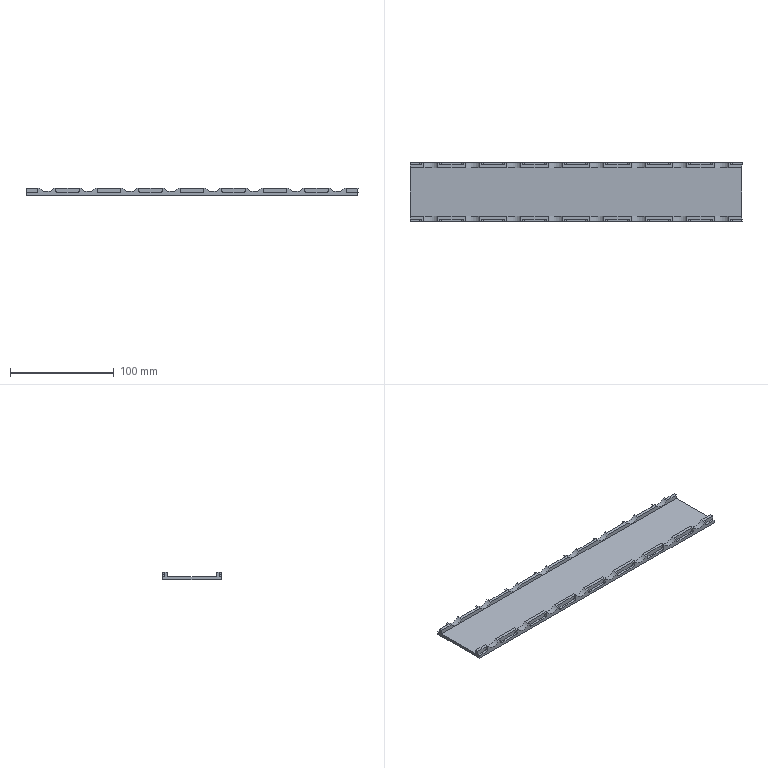NC program | Mastercam | posted with a generic post
Lines 4971 to 6130 of 9376:
(2 BM/BNOS |TOOL - 5|DIA. OFF. - 5|LEN. - 5|TOOL DIA. - 2.)
N104 T5 M6
N106 G0 G54 G90 X13.026 Y21.528 C0. B0. S6000 M3
N108 G43 H5 Z50.
N110 Z28.438
N112 Z11.438
N114 G1 Z8.438 F2000.
N116 Y21.544 Z8.246 F1000.
N118 Y21.588 Z8.058
N120 Y21.656 Z7.873
N122 Y21.745 Z7.695
N124 Y21.852 Z7.523
N126 Y21.971 Z7.36
N128 Y22.236 Z7.064
N130 X12.999 Y22.337 Z6.963
N132 X12.926 Y22.429 Z6.871
N134 X12.815 Y22.509 Z6.791
N136 X12.676 Y22.577 Z6.723
N138 X12.518 Y22.632 Z6.668
N140 X12.351 Y22.673 Z6.627
N142 X12.184 Y22.698 Z6.602
N144 X12.026 Y22.707 Z6.593
N146 X11.026
N148 X10.855
N150 X9.407
N152 X7.96
N154 X6.513
N156 X5.066
N158 X3.618
N160 X2.171
N162 X.724
N164 X-.724
N166 X-2.171
N168 X-3.618
N170 X-5.066
N172 X-6.513
N174 X-7.96
N176 X-9.407
N178 X-10.855
N180 X-12.302
N182 X-13.026
N184 X-13.057 Z6.592
N186 X-13.088 Z6.59
N188 X-13.118 Z6.586
N190 X-13.149 Z6.58
N192 X-13.179 Z6.573
N194 X-13.209 Z6.564
N196 X-13.238 Z6.554
N198 X-13.267 Z6.542
N200 X-13.295 Z6.529
N202 X-13.322 Z6.514
N204 X-13.348 Z6.498
N206 X-13.374 Z6.48
N208 X-13.398 Z6.461
N210 X-13.422 Z6.441
N212 X-13.445 Z6.42
N214 X-13.466 Z6.397
N216 X-13.599 Z6.251
N218 X-13.86 Z5.973
N220 X-14.123 Z5.717
N222 X-14.397 Z5.472
N224 X-14.681 Z5.239
N226 X-14.974 Z5.018
N228 X-15.277 Z4.81
N230 X-15.588 Z4.615
N232 X-15.907 Z4.432
N234 X-16.246 Z4.258
N236 X-16.592 Z4.099
N238 X-16.933 Z3.962
N240 X-17.279 Z3.839
N242 X-17.63 Z3.73
N244 X-17.985 Z3.637
N246 X-18.344 Z3.559
N248 X-18.706 Z3.495
N250 X-19.07 Z3.447
N252 X-19.435 Z3.415
N254 X-19.802 Z3.398
N256 X-20.184
N258 X-20.565 Z3.415
N260 X-20.93 Z3.447
N262 X-21.294 Z3.495
N264 X-21.656 Z3.559
N266 X-22.015 Z3.637
N268 X-22.37 Z3.73
N270 X-22.721 Z3.839
N272 X-23.067 Z3.962
N274 X-23.408 Z4.099
N276 X-23.754 Z4.258
N278 X-24.093 Z4.432
N280 X-24.412 Z4.615
N282 X-24.723 Z4.81
N284 X-25.026 Z5.018
N286 X-25.319 Z5.239
N288 X-25.603 Z5.472
N290 X-25.877 Z5.717
N292 X-26.14 Z5.973
N294 X-26.401 Z6.251
N296 X-26.534 Z6.397
N298 X-26.555 Z6.42
N300 X-26.578 Z6.441
N302 X-26.602 Z6.461
N304 X-26.626 Z6.48
N306 X-26.652 Z6.498
N308 X-26.678 Z6.514
N310 X-26.705 Z6.529
N312 X-26.733 Z6.542
N314 X-26.762 Z6.554
N316 X-26.791 Z6.564
N318 X-26.821 Z6.573
N320 X-26.851 Z6.58
N322 X-26.882 Z6.586
N324 X-26.912 Z6.59
N326 X-26.943 Z6.592
N328 X-26.974 Z6.593
N330 X-27.698
N332 X-29.145
N334 X-30.593
N336 X-32.04
N338 X-33.487
N340 X-34.934
N342 X-36.382
N344 X-37.829
N346 X-39.276
N348 X-40.724
N350 X-42.171
N352 X-43.618
N354 X-45.066
N356 X-46.513
N358 X-47.96
N360 X-49.407
N362 X-50.855
N364 X-52.302
N366 X-53.026
N368 X-53.057 Z6.592
N370 X-53.088 Z6.59
N372 X-53.118 Z6.586
N374 X-53.149 Z6.58
N376 X-53.179 Z6.573
N378 X-53.209 Z6.564
N380 X-53.238 Z6.554
N382 X-53.267 Z6.542
N384 X-53.295 Z6.529
N386 X-53.322 Z6.514
N388 X-53.348 Z6.498
N390 X-53.374 Z6.48
N392 X-53.398 Z6.461
N394 X-53.422 Z6.441
N396 X-53.445 Z6.42
N398 X-53.466 Z6.397
N400 X-53.599 Z6.251
N402 X-53.86 Z5.973
N404 X-54.123 Z5.717
N406 X-54.397 Z5.472
N408 X-54.681 Z5.239
N410 X-54.974 Z5.018
N412 X-55.277 Z4.81
N414 X-55.588 Z4.615
N416 X-55.907 Z4.432
N418 X-56.246 Z4.258
N420 X-56.592 Z4.099
N422 X-56.933 Z3.962
N424 X-57.279 Z3.839
N426 X-57.63 Z3.73
N428 X-57.985 Z3.637
N430 X-58.344 Z3.559
N432 X-58.706 Z3.495
N434 X-59.07 Z3.447
N436 X-59.435 Z3.415
N438 X-59.802 Z3.398
N440 X-60.184
N442 X-60.565 Z3.415
N444 X-60.93 Z3.447
N446 X-61.294 Z3.495
N448 X-61.656 Z3.559
N450 X-62.015 Z3.637
N452 X-62.37 Z3.73
N454 X-62.721 Z3.839
N456 X-63.067 Z3.962
N458 X-63.408 Z4.099
N460 X-63.754 Z4.258
N462 X-64.093 Z4.432
N464 X-64.412 Z4.615
N466 X-64.723 Z4.81
N468 X-65.026 Z5.018
N470 X-65.319 Z5.239
N472 X-65.603 Z5.472
N474 X-65.877 Z5.717
N476 X-66.14 Z5.973
N478 X-66.401 Z6.251
N480 X-66.534 Z6.397
N482 X-66.555 Z6.42
N484 X-66.578 Z6.441
N486 X-66.602 Z6.461
N488 X-66.626 Z6.48
N490 X-66.652 Z6.498
N492 X-66.678 Z6.514
N494 X-66.705 Z6.529
N496 X-66.733 Z6.542
N498 X-66.762 Z6.554
N500 X-66.791 Z6.564
N502 X-66.821 Z6.573
N504 X-66.851 Z6.58
N506 X-66.882 Z6.586
N508 X-66.912 Z6.59
N510 X-66.943 Z6.592
N512 X-66.974 Z6.593
N514 X-67.698
N516 X-69.145
N518 X-70.593
N520 X-72.04
N522 X-73.487
N524 X-74.934
N526 X-76.382
N528 X-77.829
N530 X-79.276
N532 X-80.724
N534 X-82.171
N536 X-83.618
N538 X-85.066
N540 X-86.513
N542 X-87.96
N544 X-89.407
N546 X-90.855
N548 X-92.302
N550 X-93.026
N552 X-93.057 Z6.592
N554 X-93.088 Z6.59
N556 X-93.118 Z6.586
N558 X-93.149 Z6.58
N560 X-93.179 Z6.573
N562 X-93.209 Z6.564
N564 X-93.238 Z6.554
N566 X-93.267 Z6.542
N568 X-93.295 Z6.529
N570 X-93.322 Z6.514
N572 X-93.348 Z6.498
N574 X-93.374 Z6.48
N576 X-93.398 Z6.461
N578 X-93.422 Z6.441
N580 X-93.445 Z6.42
N582 X-93.466 Z6.397
N584 X-93.599 Z6.251
N586 X-93.86 Z5.973
N588 X-94.123 Z5.717
N590 X-94.397 Z5.472
N592 X-94.681 Z5.239
N594 X-94.974 Z5.018
N596 X-95.277 Z4.81
N598 X-95.588 Z4.615
N600 X-95.907 Z4.432
N602 X-96.246 Z4.258
N604 X-96.592 Z4.099
N606 X-96.933 Z3.962
N608 X-97.279 Z3.839
N610 X-97.63 Z3.73
N612 X-97.985 Z3.637
N614 X-98.344 Z3.559
N616 X-98.706 Z3.495
N618 X-99.07 Z3.447
N620 X-99.435 Z3.415
N622 X-99.816 Z3.398
N624 X-100.198
N626 X-100.565 Z3.415
N628 X-100.93 Z3.447
N630 X-101.294 Z3.495
N632 X-101.656 Z3.559
N634 X-102.015 Z3.637
N636 X-102.37 Z3.73
N638 X-102.721 Z3.839
N640 X-103.067 Z3.962
N642 X-103.408 Z4.099
N644 X-103.754 Z4.258
N646 X-104.093 Z4.432
N648 X-104.412 Z4.615
N650 X-104.723 Z4.81
N652 X-105.026 Z5.018
N654 X-105.319 Z5.239
N656 X-105.603 Z5.472
N658 X-105.877 Z5.717
N660 X-106.14 Z5.973
N662 X-106.401 Z6.251
N664 X-106.534 Z6.397
N666 X-106.555 Z6.42
N668 X-106.578 Z6.441
N670 X-106.602 Z6.461
N672 X-106.626 Z6.48
N674 X-106.652 Z6.498
N676 X-106.678 Z6.514
N678 X-106.705 Z6.529
N680 X-106.733 Z6.542
N682 X-106.762 Z6.554
N684 X-106.791 Z6.564
N686 X-106.821 Z6.573
N688 X-106.851 Z6.58
N690 X-106.882 Z6.586
N692 X-106.912 Z6.59
N694 X-106.943 Z6.592
N696 X-106.974 Z6.593
N698 X-107.698
N700 X-109.145
N702 X-110.593
N704 X-112.04
N706 X-113.487
N708 X-114.934
N710 X-116.382
N712 X-117.829
N714 X-119.276
N716 X-120.724
N718 X-122.171
N720 X-123.618
N722 X-125.066
N724 X-126.513
N726 X-127.96
N728 X-129.408
N730 X-130.855
N732 X-132.302
N734 X-133.026
N736 X-133.057 Z6.592
N738 X-133.088 Z6.59
N740 X-133.118 Z6.586
N742 X-133.149 Z6.58
N744 X-133.179 Z6.573
N746 X-133.209 Z6.564
N748 X-133.238 Z6.554
N750 X-133.267 Z6.542
N752 X-133.295 Z6.529
N754 X-133.322 Z6.514
N756 X-133.348 Z6.498
N758 X-133.374 Z6.48
N760 X-133.398 Z6.461
N762 X-133.422 Z6.441
N764 X-133.445 Z6.42
N766 X-133.466 Z6.397
N768 X-133.599 Z6.251
N770 X-133.86 Z5.973
N772 X-134.123 Z5.717
N774 X-134.397 Z5.472
N776 X-134.681 Z5.239
N778 X-134.974 Z5.018
N780 X-135.277 Z4.81
N782 X-135.588 Z4.615
N784 X-135.907 Z4.432
N786 X-136.246 Z4.258
N788 X-136.592 Z4.099
N790 X-136.933 Z3.962
N792 X-137.279 Z3.839
N794 X-137.63 Z3.73
N796 X-137.985 Z3.637
N798 X-138.344 Z3.559
N800 X-138.706 Z3.495
N802 X-139.07 Z3.447
N804 X-139.435 Z3.415
N806 X-139.802 Z3.398
N808 X-140.184
N810 X-140.565 Z3.415
N812 X-140.93 Z3.447
N814 X-141.294 Z3.495
N816 X-141.656 Z3.559
N818 X-142.015 Z3.637
N820 X-142.37 Z3.73
N822 X-142.721 Z3.839
N824 X-143.067 Z3.962
N826 X-143.408 Z4.099
N828 X-143.754 Z4.258
N830 X-144.093 Z4.432
N832 X-144.412 Z4.615
N834 X-144.723 Z4.81
N836 X-145.026 Z5.018
N838 X-145.319 Z5.239
N840 X-145.603 Z5.472
N842 X-145.877 Z5.717
N844 X-146.14 Z5.973
N846 X-146.401 Z6.251
N848 X-146.534 Z6.397
N850 X-146.555 Z6.42
N852 X-146.578 Z6.441
N854 X-146.602 Z6.461
N856 X-146.626 Z6.48
N858 X-146.652 Z6.498
N860 X-146.678 Z6.514
N862 X-146.705 Z6.529
N864 X-146.733 Z6.542
N866 X-146.762 Z6.554
N868 X-146.791 Z6.564
N870 X-146.821 Z6.573
N872 X-146.851 Z6.58
N874 X-146.882 Z6.586
N876 X-146.912 Z6.59
N878 X-146.943 Z6.592
N880 X-146.974 Z6.593
N882 X-147.698
N884 X-149.145
N886 X-150.593
N888 X-152.04
N890 X-153.487
N892 X-154.934
N894 X-156.382
N896 X-157.829
N898 X-159.276
N900 X-160.
N902 X-160.031 Y22.708
N904 X-160.062 Y22.71
N906 X-160.093 Y22.714
N908 X-160.123 Y22.72
N910 X-160.153 Y22.727
N912 X-160.183 Y22.736
N914 X-160.213 Y22.746
N916 X-160.241 Y22.758
N918 X-160.269 Y22.772
N920 X-160.297 Y22.786
N922 X-160.323 Y22.803
N924 X-160.349 Y22.82
N926 X-160.373 Y22.839
N928 X-160.397 Y22.859
N930 X-160.419 Y22.881
N932 X-160.441 Y22.903
N934 X-160.461 Y22.927
N936 X-160.48 Y22.951
N938 X-160.497 Y22.977
N940 X-160.514 Y23.003
N942 X-160.528 Y23.031
N944 X-160.542 Y23.059
N946 X-160.554 Y23.087
N948 X-160.564 Y23.117
N950 X-160.573 Y23.147
N952 X-160.58 Y23.177
N954 X-160.586 Y23.207
N956 X-160.59 Y23.238
N958 X-160.592 Y23.269
N960 X-160.593 Y23.3
N962 Y24.
N964 Y25.4
N966 Y26.1
N968 X-160.592 Y26.131
N970 X-160.59 Y26.162
N972 X-160.586 Y26.193
N974 X-160.58 Y26.223
N976 X-160.573 Y26.253
N978 X-160.564 Y26.283
N980 X-160.554 Y26.313
N982 X-160.542 Y26.341
N984 X-160.528 Y26.369
N986 X-160.514 Y26.397
N988 X-160.497 Y26.423
N990 X-160.48 Y26.449
N992 X-160.461 Y26.473
N994 X-160.441 Y26.497
N996 X-160.419 Y26.519
N998 X-160.397 Y26.541
N1000 X-160.373 Y26.561
N1002 X-160.349 Y26.58
N1004 X-160.323 Y26.597
N1006 X-160.297 Y26.614
N1008 X-160.269 Y26.628
N1010 X-160.241 Y26.642
N1012 X-160.213 Y26.654
N1014 X-160.183 Y26.664
N1016 X-160.153 Y26.673
N1018 X-160.123 Y26.68
N1020 X-160.093 Y26.686
N1022 X-160.062 Y26.69
N1024 X-160.031 Y26.692
N1026 X-160. Y26.693
N1028 X-159.281
N1030 X-157.844
N1032 X-156.406
N1034 X-154.969
N1036 X-153.531
N1038 X-152.094
N1040 X-150.656
N1042 X-149.219
N1044 X-149.093
N1046 Y27.75
N1048 Y28.3
N1050 X-149.092 Y28.331
N1052 X-149.09 Y28.362
N1054 X-149.086 Y28.393
N1056 X-149.08 Y28.423
N1058 X-149.073 Y28.453
N1060 X-149.064 Y28.483
N1062 X-149.054 Y28.513
N1064 X-149.042 Y28.541
N1066 X-149.028 Y28.569
N1068 X-149.014 Y28.597
N1070 X-148.997 Y28.623
N1072 X-148.98 Y28.649
N1074 X-148.961 Y28.673
N1076 X-148.941 Y28.697
N1078 X-148.919 Y28.719
N1080 X-148.897 Y28.741
N1082 X-148.873 Y28.761
N1084 X-148.849 Y28.78
N1086 X-148.823 Y28.797
N1088 X-148.797 Y28.814
N1090 X-148.769 Y28.828
N1092 X-148.741 Y28.842
N1094 X-148.713 Y28.854
N1096 X-148.683 Y28.864
N1098 X-148.653 Y28.873
N1100 X-148.623 Y28.88
N1102 X-148.593 Y28.886
N1104 X-148.562 Y28.89
N1106 X-148.531 Y28.892
N1108 X-148.5 Y28.893
N1110 X-148.119
N1112 X-147.356
N1114 X-146.974
N1116 X-146.943 Z6.592
N1118 X-146.912 Z6.59
N1120 X-146.882 Z6.586
N1122 X-146.851 Z6.58
N1124 X-146.821 Z6.573
N1126 X-146.791 Z6.564
N1128 X-146.762 Z6.554
N1130 X-146.733 Z6.542
N1132 X-146.705 Z6.529
N1134 X-146.678 Z6.514
N1136 X-146.652 Z6.498
N1138 X-146.626 Z6.48
N1140 X-146.602 Z6.461
N1142 X-146.578 Z6.441
N1144 X-146.555 Z6.42
N1146 X-146.534 Z6.397
N1148 X-146.401 Z6.251
N1150 X-146.14 Z5.973
N1152 X-145.877 Z5.717
N1154 X-145.603 Z5.472
N1156 X-145.319 Z5.239
N1158 X-145.026 Z5.018
N1160 X-144.723 Z4.81
N1162 X-144.412 Z4.615
N1164 X-144.093 Z4.432
N1166 X-143.754 Z4.258
N1168 X-143.408 Z4.099
N1170 X-143.067 Z3.962
N1172 X-142.721 Z3.839
N1174 X-142.37 Z3.73
N1176 X-142.015 Z3.637
N1178 X-141.656 Z3.559
N1180 X-141.294 Z3.495
N1182 X-140.93 Z3.447
N1184 X-140.565 Z3.415
N1186 X-140.184 Z3.398
N1188 X-139.802
N1190 X-139.435 Z3.415
N1192 X-139.07 Z3.447
N1194 X-138.706 Z3.495
N1196 X-138.344 Z3.559
N1198 X-137.985 Z3.637
N1200 X-137.63 Z3.73
N1202 X-137.279 Z3.839
N1204 X-136.933 Z3.962
N1206 X-136.592 Z4.099
N1208 X-136.246 Z4.258
N1210 X-135.907 Z4.432
N1212 X-135.588 Z4.615
N1214 X-135.277 Z4.81
N1216 X-134.974 Z5.018
N1218 X-134.681 Z5.239
N1220 X-134.397 Z5.472
N1222 X-134.123 Z5.717
N1224 X-133.86 Z5.973
N1226 X-133.599 Z6.251
N1228 X-133.466 Z6.397
N1230 X-133.445 Z6.42
N1232 X-133.422 Z6.441
N1234 X-133.398 Z6.461
N1236 X-133.374 Z6.48
N1238 X-133.348 Z6.498
N1240 X-133.322 Z6.514
N1242 X-133.295 Z6.529
N1244 X-133.267 Z6.542
N1246 X-133.238 Z6.554
N1248 X-133.209 Z6.564
N1250 X-133.179 Z6.573
N1252 X-133.149 Z6.58
N1254 X-133.118 Z6.586
N1256 X-133.088 Z6.59
N1258 X-133.057 Z6.592
N1260 X-133.026 Z6.593
N1262 X-132.644
N1264 X-131.881
N1266 X-131.5
N1268 X-131.469 Y28.892
N1270 X-131.438 Y28.89
N1272 X-131.407 Y28.886
N1274 X-131.377 Y28.88
N1276 X-131.347 Y28.873
N1278 X-131.317 Y28.864
N1280 X-131.287 Y28.854
N1282 X-131.259 Y28.842
N1284 X-131.231 Y28.828
N1286 X-131.203 Y28.814
N1288 X-131.177 Y28.797
N1290 X-131.151 Y28.78
N1292 X-131.127 Y28.761
N1294 X-131.103 Y28.741
N1296 X-131.081 Y28.719
N1298 X-131.059 Y28.697
N1300 X-131.039 Y28.673
N1302 X-131.02 Y28.649
N1304 X-131.003 Y28.623
N1306 X-130.986 Y28.597
N1308 X-130.972 Y28.569
N1310 X-130.958 Y28.541
N1312 X-130.946 Y28.513
N1314 X-130.936 Y28.483
N1316 X-130.927 Y28.453
N1318 X-130.92 Y28.423
N1320 X-130.914 Y28.393
N1322 X-130.91 Y28.362
N1324 X-130.908 Y28.331
N1326 X-130.907 Y28.3
N1328 Y27.75
N1330 Y26.693
N1332 X-130.781
N1334 X-129.344
N1336 X-127.906
N1338 X-126.469
N1340 X-125.031
N1342 X-123.594
N1344 X-122.156
N1346 X-120.719
N1348 X-119.281
N1350 X-117.844
N1352 X-116.406
N1354 X-114.969
N1356 X-113.531
N1358 X-112.094
N1360 X-110.656
N1362 X-109.219
N1364 X-109.093
N1366 Y27.75
N1368 Y28.3
N1370 X-109.092 Y28.331
N1372 X-109.09 Y28.362
N1374 X-109.086 Y28.393
N1376 X-109.08 Y28.423
N1378 X-109.073 Y28.453
N1380 X-109.064 Y28.483
N1382 X-109.054 Y28.513
N1384 X-109.042 Y28.541
N1386 X-109.028 Y28.569
N1388 X-109.014 Y28.597
N1390 X-108.997 Y28.623
N1392 X-108.98 Y28.649
N1394 X-108.961 Y28.673
N1396 X-108.941 Y28.697
N1398 X-108.919 Y28.719
N1400 X-108.897 Y28.741
N1402 X-108.873 Y28.761
N1404 X-108.849 Y28.78
N1406 X-108.823 Y28.797
N1408 X-108.797 Y28.814
N1410 X-108.769 Y28.828
N1412 X-108.741 Y28.842
N1414 X-108.713 Y28.854
N1416 X-108.683 Y28.864
N1418 X-108.653 Y28.873
N1420 X-108.623 Y28.88
N1422 X-108.593 Y28.886
N1424 X-108.562 Y28.89
N1426 X-108.531 Y28.892
N1428 X-108.5 Y28.893
N1430 X-108.119
N1432 X-107.356
N1434 X-106.974
N1436 X-106.943 Z6.592
N1438 X-106.912 Z6.59
N1440 X-106.882 Z6.586
N1442 X-106.851 Z6.58
N1444 X-106.821 Z6.573
N1446 X-106.791 Z6.564
N1448 X-106.762 Z6.554
N1450 X-106.733 Z6.542
N1452 X-106.705 Z6.529
N1454 X-106.678 Z6.514
N1456 X-106.652 Z6.498
N1458 X-106.626 Z6.48
N1460 X-106.602 Z6.461
N1462 X-106.578 Z6.441
N1464 X-106.555 Z6.42
N1466 X-106.534 Z6.397
N1468 X-106.401 Z6.251
N1470 X-106.14 Z5.973
N1472 X-105.877 Z5.717
N1474 X-105.603 Z5.472
N1476 X-105.319 Z5.239
N1478 X-105.026 Z5.018
N1480 X-104.723 Z4.81
N1482 X-104.412 Z4.615
N1484 X-104.093 Z4.432
N1486 X-103.754 Z4.258
N1488 X-103.408 Z4.099
N1490 X-103.067 Z3.962
N1492 X-102.721 Z3.839
N1494 X-102.37 Z3.73
N1496 X-102.015 Z3.637
N1498 X-101.656 Z3.559
N1500 X-101.294 Z3.495
N1502 X-100.93 Z3.447
N1504 X-100.565 Z3.415
N1506 X-100.198 Z3.398
N1508 X-99.816
N1510 X-99.435 Z3.415
N1512 X-99.07 Z3.447
N1514 X-98.706 Z3.495
N1516 X-98.344 Z3.559
N1518 X-97.985 Z3.637
N1520 X-97.63 Z3.73
N1522 X-97.279 Z3.839
N1524 X-96.933 Z3.962
N1526 X-96.592 Z4.099
N1528 X-96.246 Z4.258
N1530 X-95.907 Z4.432
N1532 X-95.588 Z4.615
N1534 X-95.277 Z4.81
N1536 X-94.974 Z5.018
N1538 X-94.681 Z5.239
N1540 X-94.397 Z5.472
N1542 X-94.123 Z5.717
N1544 X-93.86 Z5.973
N1546 X-93.599 Z6.251
N1548 X-93.466 Z6.397
N1550 X-93.445 Z6.42
N1552 X-93.422 Z6.441
N1554 X-93.398 Z6.461
N1556 X-93.374 Z6.48
N1558 X-93.348 Z6.498
N1560 X-93.322 Z6.514
N1562 X-93.295 Z6.529
N1564 X-93.267 Z6.542
N1566 X-93.238 Z6.554
N1568 X-93.209 Z6.564
N1570 X-93.179 Z6.573
N1572 X-93.149 Z6.58
N1574 X-93.118 Z6.586
N1576 X-93.088 Z6.59
N1578 X-93.057 Z6.592
N1580 X-93.026 Z6.593
N1582 X-92.644
N1584 X-91.881
N1586 X-91.5
N1588 X-91.469 Y28.892
N1590 X-91.438 Y28.89
N1592 X-91.407 Y28.886
N1594 X-91.377 Y28.88
N1596 X-91.347 Y28.873
N1598 X-91.317 Y28.864
N1600 X-91.287 Y28.854
N1602 X-91.259 Y28.842
N1604 X-91.231 Y28.828
N1606 X-91.203 Y28.814
N1608 X-91.177 Y28.797
N1610 X-91.151 Y28.78
N1612 X-91.127 Y28.761
N1614 X-91.103 Y28.741
N1616 X-91.081 Y28.719
N1618 X-91.059 Y28.697
N1620 X-91.039 Y28.673
N1622 X-91.02 Y28.649
N1624 X-91.003 Y28.623
N1626 X-90.986 Y28.597
N1628 X-90.972 Y28.569
N1630 X-90.958 Y28.541
N1632 X-90.946 Y28.513
N1634 X-90.936 Y28.483
N1636 X-90.927 Y28.453
N1638 X-90.92 Y28.423
N1640 X-90.914 Y28.393
N1642 X-90.91 Y28.362
N1644 X-90.908 Y28.331
N1646 X-90.907 Y28.3
N1648 Y27.75
N1650 Y26.693
N1652 X-90.781
N1654 X-89.344
N1656 X-87.906
N1658 X-86.469
N1660 X-85.031
N1662 X-83.594
N1664 X-82.156
N1666 X-80.719
N1668 X-79.281
N1670 X-77.844
N1672 X-76.406
N1674 X-74.969
N1676 X-73.531
N1678 X-72.094
N1680 X-70.656
N1682 X-69.219
N1684 X-69.093
N1686 Y27.75
N1688 Y28.3
N1690 X-69.092 Y28.331
N1692 X-69.09 Y28.362
N1694 X-69.086 Y28.393
N1696 X-69.08 Y28.423
N1698 X-69.073 Y28.453
N1700 X-69.064 Y28.483
N1702 X-69.054 Y28.513
N1704 X-69.042 Y28.541
N1706 X-69.028 Y28.569
N1708 X-69.014 Y28.597
N1710 X-68.997 Y28.623
N1712 X-68.98 Y28.649
N1714 X-68.961 Y28.673
N1716 X-68.941 Y28.697
N1718 X-68.919 Y28.719
N1720 X-68.897 Y28.741
N1722 X-68.873 Y28.761
N1724 X-68.849 Y28.78
N1726 X-68.823 Y28.797
N1728 X-68.797 Y28.814
N1730 X-68.769 Y28.828
N1732 X-68.741 Y28.842
N1734 X-68.713 Y28.854
N1736 X-68.683 Y28.864
N1738 X-68.653 Y28.873
N1740 X-68.623 Y28.88
N1742 X-68.593 Y28.886
N1744 X-68.562 Y28.89
N1746 X-68.531 Y28.892
N1748 X-68.5 Y28.893
N1750 X-68.119
N1752 X-67.356
N1754 X-66.974
N1756 X-66.943 Z6.592
N1758 X-66.912 Z6.59
N1760 X-66.882 Z6.586
N1762 X-66.851 Z6.58
N1764 X-66.821 Z6.573
N1766 X-66.791 Z6.564
N1768 X-66.762 Z6.554
N1770 X-66.733 Z6.542
N1772 X-66.705 Z6.529
N1774 X-66.678 Z6.514
N1776 X-66.652 Z6.498
N1778 X-66.626 Z6.48
N1780 X-66.602 Z6.461
N1782 X-66.578 Z6.441
N1784 X-66.555 Z6.42
N1786 X-66.534 Z6.397
N1788 X-66.401 Z6.251
N1790 X-66.14 Z5.973
N1792 X-65.877 Z5.717
N1794 X-65.603 Z5.472
N1796 X-65.319 Z5.239
N1798 X-65.026 Z5.018
N1800 X-64.723 Z4.81
N1802 X-64.412 Z4.615
N1804 X-64.093 Z4.432
N1806 X-63.754 Z4.258
N1808 X-63.408 Z4.099
N1810 X-63.067 Z3.962
N1812 X-62.721 Z3.839
N1814 X-62.37 Z3.73
N1816 X-62.015 Z3.637
N1818 X-61.656 Z3.559
N1820 X-61.294 Z3.495
N1822 X-60.93 Z3.447
N1824 X-60.565 Z3.415
N1826 X-60.184 Z3.398
N1828 X-59.802
N1830 X-59.435 Z3.415
N1832 X-59.07 Z3.447
N1834 X-58.706 Z3.495
N1836 X-58.344 Z3.559
N1838 X-57.985 Z3.637
N1840 X-57.63 Z3.73
N1842 X-57.279 Z3.839
N1844 X-56.933 Z3.962
N1846 X-56.592 Z4.099
N1848 X-56.246 Z4.258
N1850 X-55.907 Z4.432
N1852 X-55.588 Z4.615
N1854 X-55.277 Z4.81
N1856 X-54.974 Z5.018
N1858 X-54.681 Z5.239
N1860 X-54.397 Z5.472
N1862 X-54.123 Z5.717
N1864 X-53.86 Z5.973
N1866 X-53.599 Z6.251
N1868 X-53.466 Z6.397
N1870 X-53.445 Z6.42
N1872 X-53.422 Z6.441
N1874 X-53.398 Z6.461
N1876 X-53.374 Z6.48
N1878 X-53.348 Z6.498
N1880 X-53.322 Z6.514
N1882 X-53.295 Z6.529
N1884 X-53.267 Z6.542
N1886 X-53.238 Z6.554
N1888 X-53.209 Z6.564
N1890 X-53.179 Z6.573
N1892 X-53.149 Z6.58
N1894 X-53.118 Z6.586
N1896 X-53.088 Z6.59
N1898 X-53.057 Z6.592
N1900 X-53.026 Z6.593
N1902 X-52.644
N1904 X-51.881
N1906 X-51.5
N1908 X-51.469 Y28.892
N1910 X-51.438 Y28.89
N1912 X-51.407 Y28.886
N1914 X-51.377 Y28.88
N1916 X-51.347 Y28.873
N1918 X-51.317 Y28.864
N1920 X-51.287 Y28.854
N1922 X-51.259 Y28.842
N1924 X-51.231 Y28.828
N1926 X-51.203 Y28.814
N1928 X-51.177 Y28.797
N1930 X-51.151 Y28.78
N1932 X-51.127 Y28.761
N1934 X-51.103 Y28.741
N1936 X-51.081 Y28.719
N1938 X-51.059 Y28.697
N1940 X-51.039 Y28.673
N1942 X-51.02 Y28.649
N1944 X-51.003 Y28.623
N1946 X-50.986 Y28.597
N1948 X-50.972 Y28.569
N1950 X-50.958 Y28.541
N1952 X-50.946 Y28.513
N1954 X-50.936 Y28.483
N1956 X-50.927 Y28.453
N1958 X-50.92 Y28.423
N1960 X-50.914 Y28.393
N1962 X-50.91 Y28.362
N1964 X-50.908 Y28.331
N1966 X-50.907 Y28.3
N1968 Y27.75
N1970 Y26.693
N1972 X-50.781
N1974 X-49.344
N1976 X-47.906
N1978 X-46.469
N1980 X-45.031
N1982 X-43.594
N1984 X-42.156
N1986 X-40.719
N1988 X-39.281
N1990 X-37.844
N1992 X-36.406
N1994 X-34.969
N1996 X-33.531
N1998 X-32.094
N2000 X-30.656
N2002 X-29.219
N2004 X-29.093
N2006 Y27.75
N2008 Y28.3
N2010 X-29.092 Y28.331
N2012 X-29.09 Y28.362
N2014 X-29.086 Y28.393
N2016 X-29.08 Y28.423
N2018 X-29.073 Y28.453
N2020 X-29.064 Y28.483
N2022 X-29.054 Y28.513
N2024 X-29.042 Y28.541
N2026 X-29.028 Y28.569
N2028 X-29.014 Y28.597
N2030 X-28.997 Y28.623
N2032 X-28.98 Y28.649
N2034 X-28.961 Y28.673
N2036 X-28.941 Y28.697
N2038 X-28.919 Y28.719
N2040 X-28.897 Y28.741
N2042 X-28.873 Y28.761
N2044 X-28.849 Y28.78
N2046 X-28.823 Y28.797
N2048 X-28.797 Y28.814
N2050 X-28.769 Y28.828
N2052 X-28.741 Y28.842
N2054 X-28.713 Y28.854
N2056 X-28.683 Y28.864
N2058 X-28.653 Y28.873
N2060 X-28.623 Y28.88
N2062 X-28.593 Y28.886
N2064 X-28.562 Y28.89
N2066 X-28.531 Y28.892
N2068 X-28.5 Y28.893
N2070 X-28.119
N2072 X-27.356
N2074 X-26.974
N2076 X-26.943 Z6.592
N2078 X-26.912 Z6.59
N2080 X-26.882 Z6.586
N2082 X-26.851 Z6.58
N2084 X-26.821 Z6.573
N2086 X-26.791 Z6.564
N2088 X-26.762 Z6.554
N2090 X-26.733 Z6.542
N2092 X-26.705 Z6.529
N2094 X-26.678 Z6.514
N2096 X-26.652 Z6.498
N2098 X-26.626 Z6.48
N2100 X-26.602 Z6.461
N2102 X-26.578 Z6.441
N2104 X-26.555 Z6.42
N2106 X-26.534 Z6.397
N2108 X-26.401 Z6.251
N2110 X-26.14 Z5.973
N2112 X-25.877 Z5.717
N2114 X-25.603 Z5.472
N2116 X-25.319 Z5.239
N2118 X-25.026 Z5.018
N2120 X-24.723 Z4.81
N2122 X-24.412 Z4.615
N2124 X-24.093 Z4.432
N2126 X-23.754 Z4.258
N2128 X-23.408 Z4.099
N2130 X-23.067 Z3.962
N2132 X-22.721 Z3.839
N2134 X-22.37 Z3.73
N2136 X-22.015 Z3.637
N2138 X-21.656 Z3.559
N2140 X-21.294 Z3.495
N2142 X-20.93 Z3.447
N2144 X-20.565 Z3.415
N2146 X-20.184 Z3.398
N2148 X-19.802
N2150 X-19.435 Z3.415
N2152 X-19.07 Z3.447
N2154 X-18.706 Z3.495
N2156 X-18.344 Z3.559
N2158 X-17.985 Z3.637
N2160 X-17.63 Z3.73
N2162 X-17.279 Z3.839
N2164 X-16.933 Z3.962
N2166 X-16.592 Z4.099
N2168 X-16.246 Z4.258
N2170 X-15.907 Z4.432
N2172 X-15.588 Z4.615
N2174 X-15.277 Z4.81
N2176 X-14.974 Z5.018
N2178 X-14.681 Z5.239
N2180 X-14.397 Z5.472
N2182 X-14.123 Z5.717
N2184 X-13.86 Z5.973
N2186 X-13.599 Z6.251
N2188 X-13.466 Z6.397
N2190 X-13.445 Z6.42
N2192 X-13.422 Z6.441
N2194 X-13.398 Z6.461
N2196 X-13.374 Z6.48
N2198 X-13.348 Z6.498
N2200 X-13.322 Z6.514
N2202 X-13.295 Z6.529
N2204 X-13.267 Z6.542
N2206 X-13.238 Z6.554
N2208 X-13.209 Z6.564
N2210 X-13.179 Z6.573
N2212 X-13.149 Z6.58
N2214 X-13.118 Z6.586
N2216 X-13.088 Z6.59
N2218 X-13.057 Z6.592
N2220 X-13.026 Z6.593
N2222 X-12.644
N2224 X-11.881
N2226 X-11.5
N2228 X-11.469 Y28.892
N2230 X-11.438 Y28.89
N2232 X-11.407 Y28.886
N2234 X-11.377 Y28.88
N2236 X-11.347 Y28.873
N2238 X-11.317 Y28.864
N2240 X-11.287 Y28.854
N2242 X-11.259 Y28.842
N2244 X-11.231 Y28.828
N2246 X-11.203 Y28.814
N2248 X-11.177 Y28.797
N2250 X-11.151 Y28.78
N2252 X-11.127 Y28.761
N2254 X-11.103 Y28.741
N2256 X-11.081 Y28.719
N2258 X-11.059 Y28.697
N2260 X-11.039 Y28.673
N2262 X-11.02 Y28.649
N2264 X-11.003 Y28.623
N2266 X-10.986 Y28.597
N2268 X-10.972 Y28.569
N2270 X-10.958 Y28.541
N2272 X-10.946 Y28.513
N2274 X-10.936 Y28.483
N2276 X-10.927 Y28.453
N2278 X-10.92 Y28.423
N2280 X-10.914 Y28.393
N2282 X-10.91 Y28.362
N2284 X-10.908 Y28.331
N2286 X-10.907 Y28.3
N2288 Y27.75
N2290 Y26.693
N2292 X-10.781
N2294 X-9.344
N2296 X-7.906
N2298 X-6.469
N2300 X-5.031
N2302 X-3.594
N2304 X-2.156
N2306 X-.719
N2308 X.719
N2310 X2.156
N2312 X3.594
N2314 X5.031
N2316 X6.469
N2318 X7.906
N2320 X9.344
N2322 X10.781
N2324 X10.907
N2326 Y27.75
N2328 Y28.3
N2330 X10.908 Y28.331
N2332 X10.91 Y28.362
N2334 X10.914 Y28.393
N2336 X10.92 Y28.423
N2338 X10.927 Y28.453
N2340 X10.936 Y28.483
N2342 X10.946 Y28.513
N2344 X10.958 Y28.541
N2346 X10.972 Y28.569
N2348 X10.986 Y28.597
N2350 X11.003 Y28.623
N2352 X11.02 Y28.649
N2354 X11.039 Y28.673
N2356 X11.059 Y28.697
N2358 X11.081 Y28.719
N2360 X11.103 Y28.741
N2362 X11.127 Y28.761
N2364 X11.151 Y28.78
N2366 X11.177 Y28.797
N2368 X11.203 Y28.814
N2370 X11.231 Y28.828
N2372 X11.259 Y28.842
N2374 X11.287 Y28.854
N2376 X11.317 Y28.864
N2378 X11.347 Y28.873
N2380 X11.377 Y28.88
N2382 X11.407 Y28.886
N2384 X11.438 Y28.89
N2386 X11.469 Y28.892
N2388 X11.5 Y28.893
N2390 X11.881
N2392 X12.644
N2394 X13.026
N2396 X13.057 Z6.592
N2398 X13.088 Z6.59
N2400 X13.118 Z6.586
N2402 X13.149 Z6.58
N2404 X13.179 Z6.573
N2406 X13.209 Z6.564
N2408 X13.238 Z6.554
N2410 X13.267 Z6.542
N2412 X13.295 Z6.529
N2414 X13.322 Z6.514
N2416 X13.348 Z6.498
N2418 X13.374 Z6.48
N2420 X13.398 Z6.461